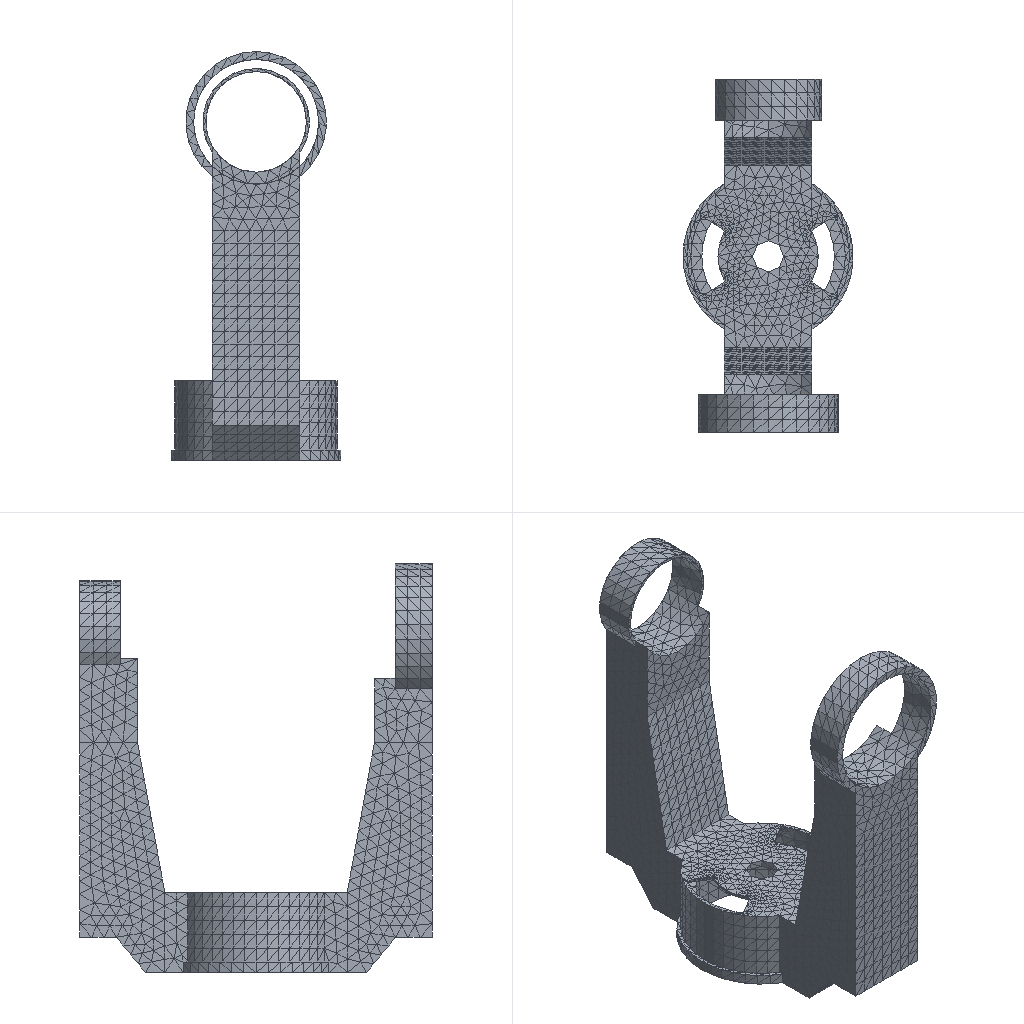Simulation study | abaqus
Set-up summary:
category,name,step,type,value,unit,region
solver,abaqus
solver,version,,,Abaqus/Standard 3DEXPERIENCE R2017x
units,not stated in the deck,,not stated
analysis,deck,,static,static
load_step,Step-1,Step-1,static,nlgeom=True
contact,interactions,,,general=0 pairs=0 ties=0
load_step,requested,,,1
mesh,nodes,,,4492
mesh,elements,,,17647
element_type,C3D4,,solid,17647
load,load commands in deck,,count,1
bc,support commands in deck,,count,6
material,MATERIAL-1,,in results
check,setup vs results,,match,"per instance, exact: element labels, types and connectivity; labels of the nodes the elements use; coordinates of those nodes at SINGLE_PRECISION in 1 of 1 instance(s)"
Results summary:
result,step,,completed,increments=11 time=1.0/1.0
result,analysis,,,static
result,last_loadstep,,,1
result,analysis steps,,count,1
result,primary field,,,U
result,reaction total,,FX,0.000539,model units
result,reaction total,,FY,0.01541,model units
result,reaction total,,FZ,13997.393,model units